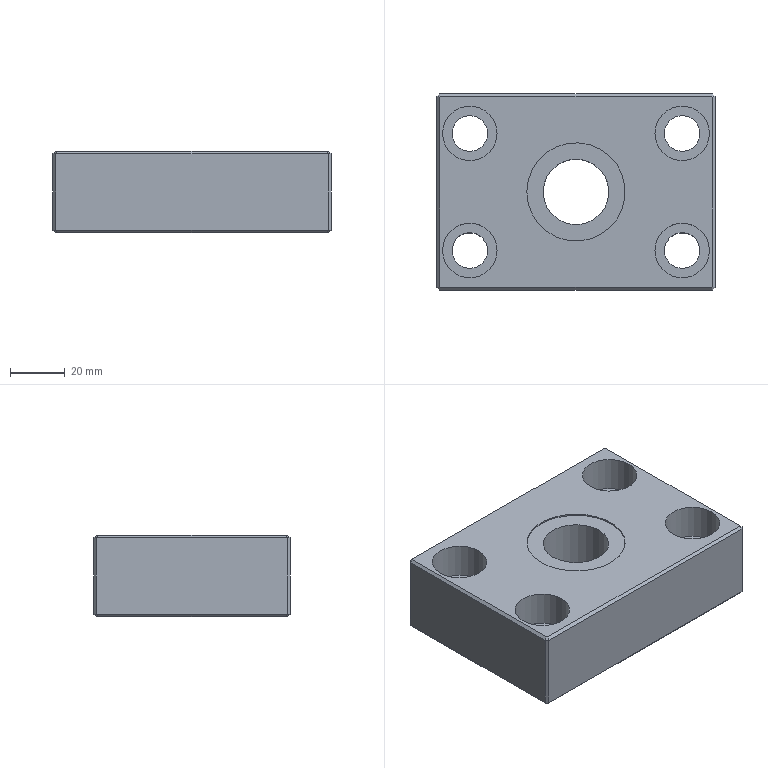Part | NX | 1 solid | 45 faces | box 102 x 72 x 30 mm | volume 178406 mm3 | plane 33 | cylinder 12 | commonest cylinder face diameters 13 x4 20 x4 24 x1 36 x1 54.5 x1 63.5 x1
STEP:
#1=CARTESIAN_POINT('',(31.75,0.,-27.25));
#2=VERTEX_POINT('',#1);
#3=CARTESIAN_POINT('',(0.,0.,-27.25));
#4=DIRECTION('',(0.,0.,-1.));
#5=DIRECTION('',(1.,0.,0.));
#6=AXIS2_PLACEMENT_3D('',#3,#4,#5);
#7=CIRCLE('',#6,31.75);
#8=EDGE_CURVE('',#2,#2,#7,.T.);
#9=ORIENTED_EDGE('',*,*,#8,.F.);
#10=EDGE_LOOP('',(#9));
#11=FACE_BOUND('',#10,.T.);
#12=CARTESIAN_POINT('',(-31.75,0.,-30.));
#13=VERTEX_POINT('',#12);
#14=CARTESIAN_POINT('',(0.,0.,-30.));
#15=DIRECTION('',(0.,0.,1.));
#16=DIRECTION('',(-1.,0.,0.));
#17=AXIS2_PLACEMENT_3D('',#14,#15,#16);
#18=CIRCLE('',#17,31.75);
#19=EDGE_CURVE('',#13,#13,#18,.T.);
#20=ORIENTED_EDGE('',*,*,#19,.F.);
#21=EDGE_LOOP('',(#20));
#22=FACE_BOUND('',#21,.T.);
#23=CARTESIAN_POINT('',(0.,0.,-27.25));
#24=DIRECTION('',(0.,0.,-1.));
#25=DIRECTION('',(-1.,0.,0.));
#26=AXIS2_PLACEMENT_3D('',#23,#24,#25);
#27=CYLINDRICAL_SURFACE('',#26,31.75);
#28=ADVANCED_FACE('',(#11,#22),#27,.F.);
#29=CARTESIAN_POINT('',(-27.25,0.,-27.25));
#30=VERTEX_POINT('',#29);
#31=CARTESIAN_POINT('',(0.,0.,-27.25));
#32=DIRECTION('',(0.,0.,-1.));
#33=DIRECTION('',(-1.,0.,0.));
#34=AXIS2_PLACEMENT_3D('',#31,#32,#33);
#35=CIRCLE('',#34,27.25);
#36=EDGE_CURVE('',#30,#30,#35,.T.);
#37=ORIENTED_EDGE('',*,*,#36,.T.);
#38=EDGE_LOOP('',(#37));
#39=FACE_BOUND('',#38,.T.);
#40=CARTESIAN_POINT('',(-27.25,0.,-30.));
#41=VERTEX_POINT('',#40);
#42=CARTESIAN_POINT('',(0.,0.,-30.));
#43=DIRECTION('',(0.,0.,1.));
#44=DIRECTION('',(-1.,0.,0.));
#45=AXIS2_PLACEMENT_3D('',#42,#43,#44);
#46=CIRCLE('',#45,27.25);
#47=EDGE_CURVE('',#41,#41,#46,.T.);
#48=ORIENTED_EDGE('',*,*,#47,.T.);
#49=EDGE_LOOP('',(#48));
#50=FACE_BOUND('',#49,.T.);
#51=CARTESIAN_POINT('',(0.,0.,-27.25));
#52=DIRECTION('',(0.,0.,-1.));
#53=DIRECTION('',(-1.,0.,0.));
#54=AXIS2_PLACEMENT_3D('',#51,#52,#53);
#55=CYLINDRICAL_SURFACE('',#54,27.25);
#56=ADVANCED_FACE('',(#39,#50),#55,.T.);
#57=ORIENTED_EDGE('',*,*,#8,.T.);
#58=EDGE_LOOP('',(#57));
#59=FACE_BOUND('',#58,.T.);
#60=ORIENTED_EDGE('',*,*,#36,.F.);
#61=EDGE_LOOP('',(#60));
#62=FACE_BOUND('',#61,.T.);
#63=CARTESIAN_POINT('',(0.,0.,-27.25));
#64=DIRECTION('',(0.,0.,-1.));
#65=DIRECTION('',(-1.,0.,0.));
#66=AXIS2_PLACEMENT_3D('',#63,#64,#65);
#67=PLANE('',#66);
#68=ADVANCED_FACE('',(#59,#62),#67,.T.);
#69=CARTESIAN_POINT('',(50.,-34.586,-30.));
#70=VERTEX_POINT('',#69);
#71=CARTESIAN_POINT('',(51.,-35.,-29.));
#72=VERTEX_POINT('',#71);
#73=CARTESIAN_POINT('',(44.324,-32.235,-35.676));
#74=DIRECTION('',(0.6786,-0.2811,0.6786));
#75=VECTOR('',#74,1000.);
#76=LINE('',#73,#75);
#77=EDGE_CURVE('',#70,#72,#76,.T.);
#78=ORIENTED_EDGE('',*,*,#77,.T.);
#79=CARTESIAN_POINT('',(50.,-36.,-29.));
#80=VERTEX_POINT('',#79);
#81=CARTESIAN_POINT('',(50.,-36.,-29.));
#82=DIRECTION('',(0.7071,0.7071,0.));
#83=VECTOR('',#82,1000.);
#84=LINE('',#81,#83);
#85=EDGE_CURVE('',#80,#72,#84,.T.);
#86=ORIENTED_EDGE('',*,*,#85,.F.);
#87=CARTESIAN_POINT('',(49.586,-35.,-30.));
#88=VERTEX_POINT('',#87);
#89=CARTESIAN_POINT('',(46.05,-26.463,-38.537));
#90=DIRECTION('',(-0.2811,0.6786,-0.6786));
#91=VECTOR('',#90,1000.);
#92=LINE('',#89,#91);
#93=EDGE_CURVE('',#80,#88,#92,.T.);
#94=ORIENTED_EDGE('',*,*,#93,.T.);
#95=CARTESIAN_POINT('',(42.293,-42.293,-30.));
#96=DIRECTION('',(-0.7071,-0.7071,0.));
#97=VECTOR('',#96,1000.);
#98=LINE('',#95,#97);
#99=EDGE_CURVE('',#70,#88,#98,.T.);
#100=ORIENTED_EDGE('',*,*,#99,.F.);
#101=EDGE_LOOP('',(#78,#86,#94,#100));
#102=FACE_BOUND('',#101,.T.);
#103=CARTESIAN_POINT('',(42.293,-42.293,-30.));
#104=DIRECTION('',(0.5,-0.5,-0.7071));
#105=DIRECTION('',(0.7071,0.7071,0.));
#106=AXIS2_PLACEMENT_3D('',#103,#104,#105);
#107=PLANE('',#106);
#108=ADVANCED_FACE('',(#102),#107,.T.);
#109=CARTESIAN_POINT('',(-50.,-36.,-29.));
#110=VERTEX_POINT('',#109);
#111=CARTESIAN_POINT('',(-49.586,-35.,-30.));
#112=VERTEX_POINT('',#111);
#113=CARTESIAN_POINT('',(-50.401,-36.967,-28.033));
#114=DIRECTION('',(0.2811,0.6786,-0.6786));
#115=VECTOR('',#114,1000.);
#116=LINE('',#113,#115);
#117=EDGE_CURVE('',#110,#112,#116,.T.);
#118=ORIENTED_EDGE('',*,*,#117,.T.);
#119=CARTESIAN_POINT('',(0.,-35.,-30.));
#120=DIRECTION('',(-1.,0.,0.));
#121=VECTOR('',#120,1000.);
#122=LINE('',#119,#121);
#123=EDGE_CURVE('',#88,#112,#122,.T.);
#124=ORIENTED_EDGE('',*,*,#123,.F.);
#125=ORIENTED_EDGE('',*,*,#93,.F.);
#126=CARTESIAN_POINT('',(0.,-36.,-29.));
#127=DIRECTION('',(1.,0.,0.));
#128=VECTOR('',#127,1000.);
#129=LINE('',#126,#128);
#130=EDGE_CURVE('',#110,#80,#129,.T.);
#131=ORIENTED_EDGE('',*,*,#130,.F.);
#132=EDGE_LOOP('',(#118,#124,#125,#131));
#133=FACE_BOUND('',#132,.T.);
#134=CARTESIAN_POINT('',(0.,-36.,-29.));
#135=DIRECTION('',(0.,0.7071,0.7071));
#136=DIRECTION('',(1.,0.,0.));
#137=AXIS2_PLACEMENT_3D('',#134,#135,#136);
#138=PLANE('',#137);
#139=ADVANCED_FACE('',(#133),#138,.F.);
#140=CARTESIAN_POINT('',(50.,34.586,-30.));
#141=VERTEX_POINT('',#140);
#142=CARTESIAN_POINT('',(51.,35.,-29.));
#143=VERTEX_POINT('',#142);
#144=CARTESIAN_POINT('',(44.324,32.235,-35.676));
#145=DIRECTION('',(0.6786,0.2811,0.6786));
#146=VECTOR('',#145,1000.);
#147=LINE('',#144,#146);
#148=EDGE_CURVE('',#141,#143,#147,.T.);
#149=ORIENTED_EDGE('',*,*,#148,.T.);
#150=CARTESIAN_POINT('',(51.,0.,-29.));
#151=DIRECTION('',(0.,1.,0.));
#152=VECTOR('',#151,1000.);
#153=LINE('',#150,#152);
#154=EDGE_CURVE('',#72,#143,#153,.T.);
#155=ORIENTED_EDGE('',*,*,#154,.F.);
#156=ORIENTED_EDGE('',*,*,#77,.F.);
#157=CARTESIAN_POINT('',(50.,0.,-30.));
#158=DIRECTION('',(0.,-1.,0.));
#159=VECTOR('',#158,1000.);
#160=LINE('',#157,#159);
#161=EDGE_CURVE('',#141,#70,#160,.T.);
#162=ORIENTED_EDGE('',*,*,#161,.F.);
#163=EDGE_LOOP('',(#149,#155,#156,#162));
#164=FACE_BOUND('',#163,.T.);
#165=CARTESIAN_POINT('',(51.,0.,-29.));
#166=DIRECTION('',(-0.7071,0.,0.7071));
#167=DIRECTION('',(0.,1.,0.));
#168=AXIS2_PLACEMENT_3D('',#165,#166,#167);
#169=PLANE('',#168);
#170=ADVANCED_FACE('',(#164),#169,.F.);
#171=CARTESIAN_POINT('',(-51.,-35.,-29.));
#172=VERTEX_POINT('',#171);
#173=CARTESIAN_POINT('',(-50.,-34.586,-30.));
#174=VERTEX_POINT('',#173);
#175=CARTESIAN_POINT('',(-44.324,-32.235,-35.676));
#176=DIRECTION('',(0.6786,0.2811,-0.6786));
#177=VECTOR('',#176,1000.);
#178=LINE('',#175,#177);
#179=EDGE_CURVE('',#172,#174,#178,.T.);
#180=ORIENTED_EDGE('',*,*,#179,.T.);
#181=CARTESIAN_POINT('',(-42.293,-42.293,-30.));
#182=DIRECTION('',(-0.7071,0.7071,0.));
#183=VECTOR('',#182,1000.);
#184=LINE('',#181,#183);
#185=EDGE_CURVE('',#112,#174,#184,.T.);
#186=ORIENTED_EDGE('',*,*,#185,.F.);
#187=ORIENTED_EDGE('',*,*,#117,.F.);
#188=CARTESIAN_POINT('',(-51.,-35.,-29.));
#189=DIRECTION('',(0.7071,-0.7071,0.));
#190=VECTOR('',#189,1000.);
#191=LINE('',#188,#190);
#192=EDGE_CURVE('',#172,#110,#191,.T.);
#193=ORIENTED_EDGE('',*,*,#192,.F.);
#194=EDGE_LOOP('',(#180,#186,#187,#193));
#195=FACE_BOUND('',#194,.T.);
#196=CARTESIAN_POINT('',(-42.293,-42.293,-30.));
#197=DIRECTION('',(-0.5,-0.5,-0.7071));
#198=DIRECTION('',(0.7071,-0.7071,0.));
#199=AXIS2_PLACEMENT_3D('',#196,#197,#198);
#200=PLANE('',#199);
#201=ADVANCED_FACE('',(#195),#200,.T.);
#202=CARTESIAN_POINT('',(49.586,35.,-30.));
#203=VERTEX_POINT('',#202);
#204=CARTESIAN_POINT('',(50.,36.,-29.));
#205=VERTEX_POINT('',#204);
#206=CARTESIAN_POINT('',(50.401,36.967,-28.033));
#207=DIRECTION('',(0.2811,0.6786,0.6786));
#208=VECTOR('',#207,1000.);
#209=LINE('',#206,#208);
#210=EDGE_CURVE('',#203,#205,#209,.T.);
#211=ORIENTED_EDGE('',*,*,#210,.T.);
#212=CARTESIAN_POINT('',(51.,35.,-29.));
#213=DIRECTION('',(-0.7071,0.7071,0.));
#214=VECTOR('',#213,1000.);
#215=LINE('',#212,#214);
#216=EDGE_CURVE('',#143,#205,#215,.T.);
#217=ORIENTED_EDGE('',*,*,#216,.F.);
#218=ORIENTED_EDGE('',*,*,#148,.F.);
#219=CARTESIAN_POINT('',(42.293,42.293,-30.));
#220=DIRECTION('',(0.7071,-0.7071,0.));
#221=VECTOR('',#220,1000.);
#222=LINE('',#219,#221);
#223=EDGE_CURVE('',#203,#141,#222,.T.);
#224=ORIENTED_EDGE('',*,*,#223,.F.);
#225=EDGE_LOOP('',(#211,#217,#218,#224));
#226=FACE_BOUND('',#225,.T.);
#227=CARTESIAN_POINT('',(42.293,42.293,-30.));
#228=DIRECTION('',(0.5,0.5,-0.7071));
#229=DIRECTION('',(-0.7071,0.7071,0.));
#230=AXIS2_PLACEMENT_3D('',#227,#228,#229);
#231=PLANE('',#230);
#232=ADVANCED_FACE('',(#226),#231,.T.);
#233=CARTESIAN_POINT('',(-51.,35.,-29.));
#234=VERTEX_POINT('',#233);
#235=CARTESIAN_POINT('',(-50.,34.586,-30.));
#236=VERTEX_POINT('',#235);
#237=CARTESIAN_POINT('',(-47.921,33.725,-32.079));
#238=DIRECTION('',(0.6786,-0.2811,-0.6786));
#239=VECTOR('',#238,1000.);
#240=LINE('',#237,#239);
#241=EDGE_CURVE('',#234,#236,#240,.T.);
#242=ORIENTED_EDGE('',*,*,#241,.T.);
#243=CARTESIAN_POINT('',(-50.,0.,-30.));
#244=DIRECTION('',(0.,1.,0.));
#245=VECTOR('',#244,1000.);
#246=LINE('',#243,#245);
#247=EDGE_CURVE('',#174,#236,#246,.T.);
#248=ORIENTED_EDGE('',*,*,#247,.F.);
#249=ORIENTED_EDGE('',*,*,#179,.F.);
#250=CARTESIAN_POINT('',(-51.,0.,-29.));
#251=DIRECTION('',(0.,-1.,0.));
#252=VECTOR('',#251,1000.);
#253=LINE('',#250,#252);
#254=EDGE_CURVE('',#234,#172,#253,.T.);
#255=ORIENTED_EDGE('',*,*,#254,.F.);
#256=EDGE_LOOP('',(#242,#248,#249,#255));
#257=FACE_BOUND('',#256,.T.);
#258=CARTESIAN_POINT('',(-51.,0.,-29.));
#259=DIRECTION('',(0.7071,0.,0.7071));
#260=DIRECTION('',(0.,-1.,0.));
#261=AXIS2_PLACEMENT_3D('',#258,#259,#260);
#262=PLANE('',#261);
#263=ADVANCED_FACE('',(#257),#262,.F.);
#264=CARTESIAN_POINT('',(-49.586,35.,-30.));
#265=VERTEX_POINT('',#264);
#266=CARTESIAN_POINT('',(-50.,36.,-29.));
#267=VERTEX_POINT('',#266);
#268=CARTESIAN_POINT('',(-46.05,26.463,-38.537));
#269=DIRECTION('',(-0.2811,0.6786,0.6786));
#270=VECTOR('',#269,1000.);
#271=LINE('',#268,#270);
#272=EDGE_CURVE('',#265,#267,#271,.T.);
#273=ORIENTED_EDGE('',*,*,#272,.T.);
#274=CARTESIAN_POINT('',(0.,36.,-29.));
#275=DIRECTION('',(-1.,0.,0.));
#276=VECTOR('',#275,1000.);
#277=LINE('',#274,#276);
#278=EDGE_CURVE('',#205,#267,#277,.T.);
#279=ORIENTED_EDGE('',*,*,#278,.F.);
#280=ORIENTED_EDGE('',*,*,#210,.F.);
#281=CARTESIAN_POINT('',(0.,35.,-30.));
#282=DIRECTION('',(1.,0.,0.));
#283=VECTOR('',#282,1000.);
#284=LINE('',#281,#283);
#285=EDGE_CURVE('',#265,#203,#284,.T.);
#286=ORIENTED_EDGE('',*,*,#285,.F.);
#287=EDGE_LOOP('',(#273,#279,#280,#286));
#288=FACE_BOUND('',#287,.T.);
#289=CARTESIAN_POINT('',(0.,36.,-29.));
#290=DIRECTION('',(0.,-0.7071,0.7071));
#291=DIRECTION('',(-1.,0.,0.));
#292=AXIS2_PLACEMENT_3D('',#289,#290,#291);
#293=PLANE('',#292);
#294=ADVANCED_FACE('',(#288),#293,.F.);
#295=ORIENTED_EDGE('',*,*,#241,.F.);
#296=CARTESIAN_POINT('',(-50.,36.,-29.));
#297=DIRECTION('',(-0.7071,-0.7071,0.));
#298=VECTOR('',#297,1000.);
#299=LINE('',#296,#298);
#300=EDGE_CURVE('',#267,#234,#299,.T.);
#301=ORIENTED_EDGE('',*,*,#300,.F.);
#302=ORIENTED_EDGE('',*,*,#272,.F.);
#303=CARTESIAN_POINT('',(-42.293,42.293,-30.));
#304=DIRECTION('',(0.7071,0.7071,0.));
#305=VECTOR('',#304,1000.);
#306=LINE('',#303,#305);
#307=EDGE_CURVE('',#236,#265,#306,.T.);
#308=ORIENTED_EDGE('',*,*,#307,.F.);
#309=EDGE_LOOP('',(#295,#301,#302,#308));
#310=FACE_BOUND('',#309,.T.);
#311=CARTESIAN_POINT('',(-42.293,42.293,-30.));
#312=DIRECTION('',(-0.5,0.5,-0.7071));
#313=DIRECTION('',(-0.7071,-0.7071,0.));
#314=AXIS2_PLACEMENT_3D('',#311,#312,#313);
#315=PLANE('',#314);
#316=ADVANCED_FACE('',(#310),#315,.T.);
#317=CARTESIAN_POINT('',(-49.586,35.,0.));
#318=VERTEX_POINT('',#317);
#319=CARTESIAN_POINT('',(-50.,36.,-1.));
#320=VERTEX_POINT('',#319);
#321=CARTESIAN_POINT('',(-46.05,26.463,8.537));
#322=DIRECTION('',(-0.2811,0.6786,-0.6786));
#323=VECTOR('',#322,1000.);
#324=LINE('',#321,#323);
#325=EDGE_CURVE('',#318,#320,#324,.T.);
#326=ORIENTED_EDGE('',*,*,#325,.T.);
#327=CARTESIAN_POINT('',(-51.,35.,-1.));
#328=VERTEX_POINT('',#327);
#329=CARTESIAN_POINT('',(-50.,36.,-1.));
#330=DIRECTION('',(0.7071,0.7071,0.));
#331=VECTOR('',#330,1000.);
#332=LINE('',#329,#331);
#333=EDGE_CURVE('',#328,#320,#332,.T.);
#334=ORIENTED_EDGE('',*,*,#333,.F.);
#335=CARTESIAN_POINT('',(-50.,34.586,0.));
#336=VERTEX_POINT('',#335);
#337=CARTESIAN_POINT('',(-44.324,32.235,5.676));
#338=DIRECTION('',(0.6786,-0.2811,0.6786));
#339=VECTOR('',#338,1000.);
#340=LINE('',#337,#339);
#341=EDGE_CURVE('',#328,#336,#340,.T.);
#342=ORIENTED_EDGE('',*,*,#341,.T.);
#343=CARTESIAN_POINT('',(-42.293,42.293,0.));
#344=DIRECTION('',(-0.7071,-0.7071,0.));
#345=VECTOR('',#344,1000.);
#346=LINE('',#343,#345);
#347=EDGE_CURVE('',#318,#336,#346,.T.);
#348=ORIENTED_EDGE('',*,*,#347,.F.);
#349=EDGE_LOOP('',(#326,#334,#342,#348));
#350=FACE_BOUND('',#349,.T.);
#351=CARTESIAN_POINT('',(-42.293,42.293,0.));
#352=DIRECTION('',(-0.5,0.5,0.7071));
#353=DIRECTION('',(0.7071,0.7071,0.));
#354=AXIS2_PLACEMENT_3D('',#351,#352,#353);
#355=PLANE('',#354);
#356=ADVANCED_FACE('',(#350),#355,.T.);
#357=CARTESIAN_POINT('',(-51.,-35.,-1.));
#358=VERTEX_POINT('',#357);
#359=CARTESIAN_POINT('',(-50.,-34.586,0.));
#360=VERTEX_POINT('',#359);
#361=CARTESIAN_POINT('',(-47.921,-33.725,2.079));
#362=DIRECTION('',(0.6786,0.2811,0.6786));
#363=VECTOR('',#362,1000.);
#364=LINE('',#361,#363);
#365=EDGE_CURVE('',#358,#360,#364,.T.);
#366=ORIENTED_EDGE('',*,*,#365,.T.);
#367=CARTESIAN_POINT('',(-50.,0.,0.));
#368=DIRECTION('',(0.,-1.,0.));
#369=VECTOR('',#368,1000.);
#370=LINE('',#367,#369);
#371=EDGE_CURVE('',#336,#360,#370,.T.);
#372=ORIENTED_EDGE('',*,*,#371,.F.);
#373=ORIENTED_EDGE('',*,*,#341,.F.);
#374=CARTESIAN_POINT('',(-51.,0.,-1.));
#375=DIRECTION('',(0.,1.,0.));
#376=VECTOR('',#375,1000.);
#377=LINE('',#374,#376);
#378=EDGE_CURVE('',#358,#328,#377,.T.);
#379=ORIENTED_EDGE('',*,*,#378,.F.);
#380=EDGE_LOOP('',(#366,#372,#373,#379));
#381=FACE_BOUND('',#380,.T.);
#382=CARTESIAN_POINT('',(-51.,0.,-1.));
#383=DIRECTION('',(0.7071,0.,-0.7071));
#384=DIRECTION('',(0.,1.,0.));
#385=AXIS2_PLACEMENT_3D('',#382,#383,#384);
#386=PLANE('',#385);
#387=ADVANCED_FACE('',(#381),#386,.F.);
#388=CARTESIAN_POINT('',(49.586,35.,0.));
#389=VERTEX_POINT('',#388);
#390=CARTESIAN_POINT('',(50.,36.,-1.));
#391=VERTEX_POINT('',#390);
#392=CARTESIAN_POINT('',(46.05,26.463,8.537));
#393=DIRECTION('',(0.2811,0.6786,-0.6786));
#394=VECTOR('',#393,1000.);
#395=LINE('',#392,#394);
#396=EDGE_CURVE('',#389,#391,#395,.T.);
#397=ORIENTED_EDGE('',*,*,#396,.T.);
#398=CARTESIAN_POINT('',(0.,36.,-1.));
#399=DIRECTION('',(1.,0.,0.));
#400=VECTOR('',#399,1000.);
#401=LINE('',#398,#400);
#402=EDGE_CURVE('',#320,#391,#401,.T.);
#403=ORIENTED_EDGE('',*,*,#402,.F.);
#404=ORIENTED_EDGE('',*,*,#325,.F.);
#405=CARTESIAN_POINT('',(0.,35.,0.));
#406=DIRECTION('',(-1.,0.,0.));
#407=VECTOR('',#406,1000.);
#408=LINE('',#405,#407);
#409=EDGE_CURVE('',#389,#318,#408,.T.);
#410=ORIENTED_EDGE('',*,*,#409,.F.);
#411=EDGE_LOOP('',(#397,#403,#404,#410));
#412=FACE_BOUND('',#411,.T.);
#413=CARTESIAN_POINT('',(0.,36.,-1.));
#414=DIRECTION('',(0.,-0.7071,-0.7071));
#415=DIRECTION('',(1.,0.,0.));
#416=AXIS2_PLACEMENT_3D('',#413,#414,#415);
#417=PLANE('',#416);
#418=ADVANCED_FACE('',(#412),#417,.F.);
#419=CARTESIAN_POINT('',(-50.,-36.,-1.));
#420=VERTEX_POINT('',#419);
#421=CARTESIAN_POINT('',(-49.586,-35.,0.));
#422=VERTEX_POINT('',#421);
#423=CARTESIAN_POINT('',(-46.05,-26.463,8.537));
#424=DIRECTION('',(0.2811,0.6786,0.6786));
#425=VECTOR('',#424,1000.);
#426=LINE('',#423,#425);
#427=EDGE_CURVE('',#420,#422,#426,.T.);
#428=ORIENTED_EDGE('',*,*,#427,.T.);
#429=CARTESIAN_POINT('',(-42.293,-42.293,0.));
#430=DIRECTION('',(0.7071,-0.7071,0.));
#431=VECTOR('',#430,1000.);
#432=LINE('',#429,#431);
#433=EDGE_CURVE('',#360,#422,#432,.T.);
#434=ORIENTED_EDGE('',*,*,#433,.F.);
#435=ORIENTED_EDGE('',*,*,#365,.F.);
#436=CARTESIAN_POINT('',(-51.,-35.,-1.));
#437=DIRECTION('',(-0.7071,0.7071,0.));
#438=VECTOR('',#437,1000.);
#439=LINE('',#436,#438);
#440=EDGE_CURVE('',#420,#358,#439,.T.);
#441=ORIENTED_EDGE('',*,*,#440,.F.);
#442=EDGE_LOOP('',(#428,#434,#435,#441));
#443=FACE_BOUND('',#442,.T.);
#444=CARTESIAN_POINT('',(-42.293,-42.293,0.));
#445=DIRECTION('',(-0.5,-0.5,0.7071));
#446=DIRECTION('',(-0.7071,0.7071,0.));
#447=AXIS2_PLACEMENT_3D('',#444,#445,#446);
#448=PLANE('',#447);
#449=ADVANCED_FACE('',(#443),#448,.T.);
#450=CARTESIAN_POINT('',(50.,34.586,0.));
#451=VERTEX_POINT('',#450);
#452=CARTESIAN_POINT('',(51.,35.,-1.));
#453=VERTEX_POINT('',#452);
#454=CARTESIAN_POINT('',(47.921,33.725,2.079));
#455=DIRECTION('',(0.6786,0.2811,-0.6786));
#456=VECTOR('',#455,1000.);
#457=LINE('',#454,#456);
#458=EDGE_CURVE('',#451,#453,#457,.T.);
#459=ORIENTED_EDGE('',*,*,#458,.T.);
#460=CARTESIAN_POINT('',(51.,35.,-1.));
#461=DIRECTION('',(0.7071,-0.7071,0.));
#462=VECTOR('',#461,1000.);
#463=LINE('',#460,#462);
#464=EDGE_CURVE('',#391,#453,#463,.T.);
#465=ORIENTED_EDGE('',*,*,#464,.F.);
#466=ORIENTED_EDGE('',*,*,#396,.F.);
#467=CARTESIAN_POINT('',(42.293,42.293,0.));
#468=DIRECTION('',(-0.7071,0.7071,0.));
#469=VECTOR('',#468,1000.);
#470=LINE('',#467,#469);
#471=EDGE_CURVE('',#451,#389,#470,.T.);
#472=ORIENTED_EDGE('',*,*,#471,.F.);
#473=EDGE_LOOP('',(#459,#465,#466,#472));
#474=FACE_BOUND('',#473,.T.);
#475=CARTESIAN_POINT('',(42.293,42.293,0.));
#476=DIRECTION('',(0.5,0.5,0.7071));
#477=DIRECTION('',(0.7071,-0.7071,0.));
#478=AXIS2_PLACEMENT_3D('',#475,#476,#477);
#479=PLANE('',#478);
#480=ADVANCED_FACE('',(#474),#479,.T.);
#481=CARTESIAN_POINT('',(50.,-36.,-1.));
#482=VERTEX_POINT('',#481);
#483=CARTESIAN_POINT('',(49.586,-35.,0.));
#484=VERTEX_POINT('',#483);
#485=CARTESIAN_POINT('',(50.401,-36.967,-1.967));
#486=DIRECTION('',(-0.2811,0.6786,0.6786));
#487=VECTOR('',#486,1000.);
#488=LINE('',#485,#487);
#489=EDGE_CURVE('',#482,#484,#488,.T.);
#490=ORIENTED_EDGE('',*,*,#489,.T.);
#491=CARTESIAN_POINT('',(0.,-35.,0.));
#492=DIRECTION('',(1.,0.,0.));
#493=VECTOR('',#492,1000.);
#494=LINE('',#491,#493);
#495=EDGE_CURVE('',#422,#484,#494,.T.);
#496=ORIENTED_EDGE('',*,*,#495,.F.);
#497=ORIENTED_EDGE('',*,*,#427,.F.);
#498=CARTESIAN_POINT('',(0.,-36.,-1.));
#499=DIRECTION('',(-1.,0.,0.));
#500=VECTOR('',#499,1000.);
#501=LINE('',#498,#500);
#502=EDGE_CURVE('',#482,#420,#501,.T.);
#503=ORIENTED_EDGE('',*,*,#502,.F.);
#504=EDGE_LOOP('',(#490,#496,#497,#503));
#505=FACE_BOUND('',#504,.T.);
#506=CARTESIAN_POINT('',(0.,-36.,-1.));
#507=DIRECTION('',(0.,0.7071,-0.7071));
#508=DIRECTION('',(-1.,0.,0.));
#509=AXIS2_PLACEMENT_3D('',#506,#507,#508);
#510=PLANE('',#509);
#511=ADVANCED_FACE('',(#505),#510,.F.);
#512=CARTESIAN_POINT('',(50.,-34.586,0.));
#513=VERTEX_POINT('',#512);
#514=CARTESIAN_POINT('',(51.,-35.,-1.));
#515=VERTEX_POINT('',#514);
#516=CARTESIAN_POINT('',(44.324,-32.235,5.676));
#517=DIRECTION('',(0.6786,-0.2811,-0.6786));
#518=VECTOR('',#517,1000.);
#519=LINE('',#516,#518);
#520=EDGE_CURVE('',#513,#515,#519,.T.);
#521=ORIENTED_EDGE('',*,*,#520,.T.);
#522=CARTESIAN_POINT('',(51.,0.,-1.));
#523=DIRECTION('',(0.,-1.,0.));
#524=VECTOR('',#523,1000.);
#525=LINE('',#522,#524);
#526=EDGE_CURVE('',#453,#515,#525,.T.);
#527=ORIENTED_EDGE('',*,*,#526,.F.);
#528=ORIENTED_EDGE('',*,*,#458,.F.);
#529=CARTESIAN_POINT('',(50.,0.,0.));
#530=DIRECTION('',(0.,1.,0.));
#531=VECTOR('',#530,1000.);
#532=LINE('',#529,#531);
#533=EDGE_CURVE('',#513,#451,#532,.T.);
#534=ORIENTED_EDGE('',*,*,#533,.F.);
#535=EDGE_LOOP('',(#521,#527,#528,#534));
#536=FACE_BOUND('',#535,.T.);
#537=CARTESIAN_POINT('',(51.,0.,-1.));
#538=DIRECTION('',(-0.7071,0.,-0.7071));
#539=DIRECTION('',(0.,-1.,0.));
#540=AXIS2_PLACEMENT_3D('',#537,#538,#539);
#541=PLANE('',#540);
#542=ADVANCED_FACE('',(#536),#541,.F.);
#543=ORIENTED_EDGE('',*,*,#489,.F.);
#544=CARTESIAN_POINT('',(50.,-36.,-1.));
#545=DIRECTION('',(-0.7071,-0.7071,0.));
#546=VECTOR('',#545,1000.);
#547=LINE('',#544,#546);
#548=EDGE_CURVE('',#515,#482,#547,.T.);
#549=ORIENTED_EDGE('',*,*,#548,.F.);
#550=ORIENTED_EDGE('',*,*,#520,.F.);
#551=CARTESIAN_POINT('',(42.293,-42.293,0.));
#552=DIRECTION('',(0.7071,0.7071,0.));
#553=VECTOR('',#552,1000.);
#554=LINE('',#551,#553);
#555=EDGE_CURVE('',#484,#513,#554,.T.);
#556=ORIENTED_EDGE('',*,*,#555,.F.);
#557=EDGE_LOOP('',(#543,#549,#550,#556));
#558=FACE_BOUND('',#557,.T.);
#559=CARTESIAN_POINT('',(42.293,-42.293,0.));
#560=DIRECTION('',(0.5,-0.5,0.7071));
#561=DIRECTION('',(-0.7071,-0.7071,0.));
#562=AXIS2_PLACEMENT_3D('',#559,#560,#561);
#563=PLANE('',#562);
#564=ADVANCED_FACE('',(#558),#563,.T.);
#565=CARTESIAN_POINT('',(50.,-36.,-30.));
#566=DIRECTION('',(0.,0.,1.));
#567=VECTOR('',#566,1000.);
#568=LINE('',#565,#567);
#569=EDGE_CURVE('',#80,#482,#568,.T.);
#570=ORIENTED_EDGE('',*,*,#569,.F.);
#571=ORIENTED_EDGE('',*,*,#85,.T.);
#572=CARTESIAN_POINT('',(51.,-35.,-30.));
#573=DIRECTION('',(0.,0.,-1.));
#574=VECTOR('',#573,1000.);
#575=LINE('',#572,#574);
#576=EDGE_CURVE('',#515,#72,#575,.T.);
#577=ORIENTED_EDGE('',*,*,#576,.F.);
#578=ORIENTED_EDGE('',*,*,#548,.T.);
#579=EDGE_LOOP('',(#570,#571,#577,#578));
#580=FACE_BOUND('',#579,.T.);
#581=CARTESIAN_POINT('',(50.,-36.,-30.));
#582=DIRECTION('',(-0.7071,0.7071,0.));
#583=DIRECTION('',(0.,0.,1.));
#584=AXIS2_PLACEMENT_3D('',#581,#582,#583);
#585=PLANE('',#584);
#586=ADVANCED_FACE('',(#580),#585,.F.);
#587=CARTESIAN_POINT('',(-51.,-35.,-30.));
#588=DIRECTION('',(0.,0.,1.));
#589=VECTOR('',#588,1000.);
#590=LINE('',#587,#589);
#591=EDGE_CURVE('',#172,#358,#590,.T.);
#592=ORIENTED_EDGE('',*,*,#591,.F.);
#593=ORIENTED_EDGE('',*,*,#192,.T.);
#594=CARTESIAN_POINT('',(-50.,-36.,-30.));
#595=DIRECTION('',(0.,0.,-1.));
#596=VECTOR('',#595,1000.);
#597=LINE('',#594,#596);
#598=EDGE_CURVE('',#420,#110,#597,.T.);
#599=ORIENTED_EDGE('',*,*,#598,.F.);
#600=ORIENTED_EDGE('',*,*,#440,.T.);
#601=EDGE_LOOP('',(#592,#593,#599,#600));
#602=FACE_BOUND('',#601,.T.);
#603=CARTESIAN_POINT('',(-51.,-35.,-30.));
#604=DIRECTION('',(0.7071,0.7071,0.));
#605=DIRECTION('',(0.,0.,1.));
#606=AXIS2_PLACEMENT_3D('',#603,#604,#605);
#607=PLANE('',#606);
#608=ADVANCED_FACE('',(#602),#607,.F.);
#609=CARTESIAN_POINT('',(51.,35.,-30.));
#610=DIRECTION('',(0.,0.,1.));
#611=VECTOR('',#610,1000.);
#612=LINE('',#609,#611);
#613=EDGE_CURVE('',#143,#453,#612,.T.);
#614=ORIENTED_EDGE('',*,*,#613,.F.);
#615=ORIENTED_EDGE('',*,*,#216,.T.);
#616=CARTESIAN_POINT('',(50.,36.,-30.));
#617=DIRECTION('',(0.,0.,-1.));
#618=VECTOR('',#617,1000.);
#619=LINE('',#616,#618);
#620=EDGE_CURVE('',#391,#205,#619,.T.);
#621=ORIENTED_EDGE('',*,*,#620,.F.);
#622=ORIENTED_EDGE('',*,*,#464,.T.);
#623=EDGE_LOOP('',(#614,#615,#621,#622));
#624=FACE_BOUND('',#623,.T.);
#625=CARTESIAN_POINT('',(51.,35.,-30.));
#626=DIRECTION('',(-0.7071,-0.7071,0.));
#627=DIRECTION('',(0.,0.,1.));
#628=AXIS2_PLACEMENT_3D('',#625,#626,#627);
#629=PLANE('',#628);
#630=ADVANCED_FACE('',(#624),#629,.F.);
#631=CARTESIAN_POINT('',(-50.,36.,-30.));
#632=DIRECTION('',(0.,0.,1.));
#633=VECTOR('',#632,1000.);
#634=LINE('',#631,#633);
#635=EDGE_CURVE('',#267,#320,#634,.T.);
#636=ORIENTED_EDGE('',*,*,#635,.F.);
#637=ORIENTED_EDGE('',*,*,#300,.T.);
#638=CARTESIAN_POINT('',(-51.,35.,-30.));
#639=DIRECTION('',(0.,0.,-1.));
#640=VECTOR('',#639,1000.);
#641=LINE('',#638,#640);
#642=EDGE_CURVE('',#328,#234,#641,.T.);
#643=ORIENTED_EDGE('',*,*,#642,.F.);
#644=ORIENTED_EDGE('',*,*,#333,.T.);
#645=EDGE_LOOP('',(#636,#637,#643,#644));
#646=FACE_BOUND('',#645,.T.);
#647=CARTESIAN_POINT('',(-50.,36.,-30.));
#648=DIRECTION('',(0.7071,-0.7071,0.));
#649=DIRECTION('',(0.,0.,1.));
#650=AXIS2_PLACEMENT_3D('',#647,#648,#649);
#651=PLANE('',#650);
#652=ADVANCED_FACE('',(#646),#651,.F.);
#653=CARTESIAN_POINT('',(-18.,0.,0.));
#654=VERTEX_POINT('',#653);
#655=CARTESIAN_POINT('',(0.,0.,0.));
#656=DIRECTION('',(0.,0.,-1.));
#657=DIRECTION('',(-1.,0.,0.));
#658=AXIS2_PLACEMENT_3D('',#655,#656,#657);
#659=CIRCLE('',#658,18.);
#660=EDGE_CURVE('',#654,#654,#659,.T.);
#661=ORIENTED_EDGE('',*,*,#660,.F.);
#662=EDGE_LOOP('',(#661));
#663=FACE_BOUND('',#662,.T.);
#664=CARTESIAN_POINT('',(-18.,0.,-0.5));
#665=VERTEX_POINT('',#664);
#666=CARTESIAN_POINT('',(0.,0.,-0.5));
#667=DIRECTION('',(0.,0.,1.));
#668=DIRECTION('',(-1.,0.,0.));
#669=AXIS2_PLACEMENT_3D('',#666,#667,#668);
#670=CIRCLE('',#669,18.);
#671=EDGE_CURVE('',#665,#665,#670,.T.);
#672=ORIENTED_EDGE('',*,*,#671,.F.);
#673=EDGE_LOOP('',(#672));
#674=FACE_BOUND('',#673,.T.);
#675=CARTESIAN_POINT('',(0.,0.,0.));
#676=DIRECTION('',(0.,0.,-1.));
#677=DIRECTION('',(-1.,0.,0.));
#678=AXIS2_PLACEMENT_3D('',#675,#676,#677);
#679=CYLINDRICAL_SURFACE('',#678,18.);
#680=ADVANCED_FACE('',(#663,#674),#679,.F.);
#681=ORIENTED_EDGE('',*,*,#671,.T.);
#682=EDGE_LOOP('',(#681));
#683=FACE_BOUND('',#682,.T.);
#684=CARTESIAN_POINT('',(-12.,0.,-0.5));
#685=VERTEX_POINT('',#684);
#686=CARTESIAN_POINT('',(0.,0.,-0.5));
#687=DIRECTION('',(0.,0.,1.));
#688=DIRECTION('',(-1.,0.,0.));
#689=AXIS2_PLACEMENT_3D('',#686,#687,#688);
#690=CIRCLE('',#689,12.);
#691=EDGE_CURVE('',#685,#685,#690,.T.);
#692=ORIENTED_EDGE('',*,*,#691,.F.);
#693=EDGE_LOOP('',(#692));
#694=FACE_BOUND('',#693,.T.);
#695=CARTESIAN_POINT('',(0.,0.,-0.5));
#696=DIRECTION('',(0.,0.,-1.));
#697=DIRECTION('',(-1.,0.,0.));
#698=AXIS2_PLACEMENT_3D('',#695,#696,#697);
#699=PLANE('',#698);
#700=ADVANCED_FACE('',(#683,#694),#699,.F.);
#701=ORIENTED_EDGE('',*,*,#691,.T.);
#702=EDGE_LOOP('',(#701));
#703=FACE_BOUND('',#702,.T.);
#704=CARTESIAN_POINT('',(-12.,0.,-30.));
#705=VERTEX_POINT('',#704);
#706=CARTESIAN_POINT('',(0.,0.,-30.));
#707=DIRECTION('',(0.,0.,-1.));
#708=DIRECTION('',(-1.,0.,0.));
#709=AXIS2_PLACEMENT_3D('',#706,#707,#708);
#710=CIRCLE('',#709,12.);
#711=EDGE_CURVE('',#705,#705,#710,.T.);
#712=ORIENTED_EDGE('',*,*,#711,.T.);
#713=EDGE_LOOP('',(#712));
#714=FACE_BOUND('',#713,.T.);
#715=CARTESIAN_POINT('',(0.,0.,-50.));
#716=DIRECTION('',(0.,0.,-1.));
#717=DIRECTION('',(-1.,0.,0.));
#718=AXIS2_PLACEMENT_3D('',#715,#716,#717);
#719=CYLINDRICAL_SURFACE('',#718,12.);
#720=ADVANCED_FACE('',(#703,#714),#719,.F.);
#721=CARTESIAN_POINT('',(-48.9,21.45,0.));
#722=VERTEX_POINT('',#721);
#723=CARTESIAN_POINT('',(-38.9,21.45,0.));
#724=DIRECTION('',(0.,0.,-1.));
#725=DIRECTION('',(-1.,0.,0.));
#726=AXIS2_PLACEMENT_3D('',#723,#724,#725);
#727=CIRCLE('',#726,10.);
#728=EDGE_CURVE('',#722,#722,#727,.T.);
#729=ORIENTED_EDGE('',*,*,#728,.F.);
#730=EDGE_LOOP('',(#729));
#731=FACE_BOUND('',#730,.T.);
#732=CARTESIAN_POINT('',(-48.9,21.45,-13.));
#733=VERTEX_POINT('',#732);
#734=CARTESIAN_POINT('',(-38.9,21.45,-13.));
#735=DIRECTION('',(0.,0.,1.));
#736=DIRECTION('',(-1.,0.,0.));
#737=AXIS2_PLACEMENT_3D('',#734,#735,#736);
#738=CIRCLE('',#737,10.);
#739=EDGE_CURVE('',#733,#733,#738,.T.);
#740=ORIENTED_EDGE('',*,*,#739,.F.);
#741=EDGE_LOOP('',(#740));
#742=FACE_BOUND('',#741,.T.);
#743=CARTESIAN_POINT('',(-38.9,21.45,0.));
#744=DIRECTION('',(0.,0.,-1.));
#745=DIRECTION('',(-1.,0.,0.));
#746=AXIS2_PLACEMENT_3D('',#743,#744,#745);
#747=CYLINDRICAL_SURFACE('',#746,10.);
#748=ADVANCED_FACE('',(#731,#742),#747,.F.);
#749=ORIENTED_EDGE('',*,*,#739,.T.);
#750=EDGE_LOOP('',(#749));
#751=FACE_BOUND('',#750,.T.);
#752=CARTESIAN_POINT('',(-45.4,21.45,-13.));
#753=VERTEX_POINT('',#752);
#754=CARTESIAN_POINT('',(-38.9,21.45,-13.));
#755=DIRECTION('',(0.,0.,1.));
#756=DIRECTION('',(-1.,0.,0.));
#757=AXIS2_PLACEMENT_3D('',#754,#755,#756);
#758=CIRCLE('',#757,6.5);
#759=EDGE_CURVE('',#753,#753,#758,.T.);
#760=ORIENTED_EDGE('',*,*,#759,.F.);
#761=EDGE_LOOP('',(#760));
#762=FACE_BOUND('',#761,.T.);
#763=CARTESIAN_POINT('',(-38.9,21.45,-13.));
#764=DIRECTION('',(0.,0.,-1.));
#765=DIRECTION('',(-1.,0.,0.));
#766=AXIS2_PLACEMENT_3D('',#763,#764,#765);
#767=PLANE('',#766);
#768=ADVANCED_FACE('',(#751,#762),#767,.F.);
#769=ORIENTED_EDGE('',*,*,#759,.T.);
#770=EDGE_LOOP('',(#769));
#771=FACE_BOUND('',#770,.T.);
#772=CARTESIAN_POINT('',(-45.4,21.45,-30.));
#773=VERTEX_POINT('',#772);
#774=CARTESIAN_POINT('',(-38.9,21.45,-30.));
#775=DIRECTION('',(0.,0.,-1.));
#776=DIRECTION('',(-1.,0.,0.));
#777=AXIS2_PLACEMENT_3D('',#774,#775,#776);
#778=CIRCLE('',#777,6.5);
#779=EDGE_CURVE('',#773,#773,#778,.T.);
#780=ORIENTED_EDGE('',*,*,#779,.T.);
#781=EDGE_LOOP('',(#780));
#782=FACE_BOUND('',#781,.T.);
#783=CARTESIAN_POINT('',(-38.9,21.45,-50.));
#784=DIRECTION('',(0.,0.,-1.));
#785=DIRECTION('',(-1.,0.,0.));
#786=AXIS2_PLACEMENT_3D('',#783,#784,#785);
#787=CYLINDRICAL_SURFACE('',#786,6.5);
#788=ADVANCED_FACE('',(#771,#782),#787,.F.);
#789=ORIENTED_EDGE('',*,*,#576,.T.);
#790=ORIENTED_EDGE('',*,*,#154,.T.);
#791=ORIENTED_EDGE('',*,*,#613,.T.);
#792=ORIENTED_EDGE('',*,*,#526,.T.);
#793=EDGE_LOOP('',(#789,#790,#791,#792));
#794=FACE_BOUND('',#793,.T.);
#795=CARTESIAN_POINT('',(51.,0.,-30.));
#796=DIRECTION('',(1.,0.,0.));
#797=DIRECTION('',(0.,0.,-1.));
#798=AXIS2_PLACEMENT_3D('',#795,#796,#797);
#799=PLANE('',#798);
#800=ADVANCED_FACE('',(#794),#799,.T.);
#801=ORIENTED_EDGE('',*,*,#779,.F.);
#802=EDGE_LOOP('',(#801));
#803=FACE_BOUND('',#802,.T.);
#804=CARTESIAN_POINT('',(-45.4,-21.45,-30.));
#805=VERTEX_POINT('',#804);
#806=CARTESIAN_POINT('',(-38.9,-21.45,-30.));
#807=DIRECTION('',(0.,0.,-1.));
#808=DIRECTION('',(-1.,0.,0.));
#809=AXIS2_PLACEMENT_3D('',#806,#807,#808);
#810=CIRCLE('',#809,6.5);
#811=EDGE_CURVE('',#805,#805,#810,.T.);
#812=ORIENTED_EDGE('',*,*,#811,.F.);
#813=EDGE_LOOP('',(#812));
#814=FACE_BOUND('',#813,.T.);
#815=CARTESIAN_POINT('',(32.4,-21.45,-30.));
#816=VERTEX_POINT('',#815);
#817=CARTESIAN_POINT('',(38.9,-21.45,-30.));
#818=DIRECTION('',(0.,0.,-1.));
#819=DIRECTION('',(-1.,0.,0.));
#820=AXIS2_PLACEMENT_3D('',#817,#818,#819);
#821=CIRCLE('',#820,6.5);
#822=EDGE_CURVE('',#816,#816,#821,.T.);
#823=ORIENTED_EDGE('',*,*,#822,.F.);
#824=EDGE_LOOP('',(#823));
#825=FACE_BOUND('',#824,.T.);
#826=CARTESIAN_POINT('',(32.4,21.45,-30.));
#827=VERTEX_POINT('',#826);
#828=CARTESIAN_POINT('',(38.9,21.45,-30.));
#829=DIRECTION('',(0.,0.,-1.));
#830=DIRECTION('',(-1.,0.,0.));
#831=AXIS2_PLACEMENT_3D('',#828,#829,#830);
#832=CIRCLE('',#831,6.5);
#833=EDGE_CURVE('',#827,#827,#832,.T.);
#834=ORIENTED_EDGE('',*,*,#833,.F.);
#835=EDGE_LOOP('',(#834));
#836=FACE_BOUND('',#835,.T.);
#837=ORIENTED_EDGE('',*,*,#161,.T.);
#838=ORIENTED_EDGE('',*,*,#99,.T.);
#839=ORIENTED_EDGE('',*,*,#123,.T.);
#840=ORIENTED_EDGE('',*,*,#185,.T.);
#841=ORIENTED_EDGE('',*,*,#247,.T.);
#842=ORIENTED_EDGE('',*,*,#307,.T.);
#843=ORIENTED_EDGE('',*,*,#285,.T.);
#844=ORIENTED_EDGE('',*,*,#223,.T.);
#845=EDGE_LOOP('',(#837,#838,#839,#840,#841,#842,#843,#844));
#846=FACE_BOUND('',#845,.T.);
#847=ORIENTED_EDGE('',*,*,#19,.T.);
#848=EDGE_LOOP('',(#847));
#849=FACE_BOUND('',#848,.T.);
#850=CARTESIAN_POINT('',(0.,0.,-30.));
#851=DIRECTION('',(0.,0.,-1.));
#852=DIRECTION('',(-1.,0.,0.));
#853=AXIS2_PLACEMENT_3D('',#850,#851,#852);
#854=PLANE('',#853);
#855=ADVANCED_FACE('',(#803,#814,#825,#836,#846,#849),#854,.T.);
#856=ORIENTED_EDGE('',*,*,#620,.T.);
#857=ORIENTED_EDGE('',*,*,#278,.T.);
#858=ORIENTED_EDGE('',*,*,#635,.T.);
#859=ORIENTED_EDGE('',*,*,#402,.T.);
#860=EDGE_LOOP('',(#856,#857,#858,#859));
#861=FACE_BOUND('',#860,.T.);
#862=CARTESIAN_POINT('',(0.,36.,-30.));
#863=DIRECTION('',(0.,1.,0.));
#864=DIRECTION('',(0.,0.,1.));
#865=AXIS2_PLACEMENT_3D('',#862,#863,#864);
#866=PLANE('',#865);
#867=ADVANCED_FACE('',(#861),#866,.T.);
#868=ORIENTED_EDGE('',*,*,#642,.T.);
#869=ORIENTED_EDGE('',*,*,#254,.T.);
#870=ORIENTED_EDGE('',*,*,#591,.T.);
#871=ORIENTED_EDGE('',*,*,#378,.T.);
#872=EDGE_LOOP('',(#868,#869,#870,#871));
#873=FACE_BOUND('',#872,.T.);
#874=CARTESIAN_POINT('',(-51.,0.,-30.));
#875=DIRECTION('',(-1.,0.,0.));
#876=DIRECTION('',(0.,0.,1.));
#877=AXIS2_PLACEMENT_3D('',#874,#875,#876);
#878=PLANE('',#877);
#879=ADVANCED_FACE('',(#873),#878,.T.);
#880=ORIENTED_EDGE('',*,*,#598,.T.);
#881=ORIENTED_EDGE('',*,*,#130,.T.);
#882=ORIENTED_EDGE('',*,*,#569,.T.);
#883=ORIENTED_EDGE('',*,*,#502,.T.);
#884=EDGE_LOOP('',(#880,#881,#882,#883));
#885=FACE_BOUND('',#884,.T.);
#886=CARTESIAN_POINT('',(0.,-36.,-30.));
#887=DIRECTION('',(0.,-1.,0.));
#888=DIRECTION('',(0.,0.,-1.));
#889=AXIS2_PLACEMENT_3D('',#886,#887,#888);
#890=PLANE('',#889);
#891=ADVANCED_FACE('',(#885),#890,.T.);
#892=ORIENTED_EDGE('',*,*,#728,.T.);
#893=EDGE_LOOP('',(#892));
#894=FACE_BOUND('',#893,.T.);
#895=CARTESIAN_POINT('',(-48.9,-21.45,0.));
#896=VERTEX_POINT('',#895);
#897=CARTESIAN_POINT('',(-38.9,-21.45,0.));
#898=DIRECTION('',(0.,0.,-1.));
#899=DIRECTION('',(-1.,0.,0.));
#900=AXIS2_PLACEMENT_3D('',#897,#898,#899);
#901=CIRCLE('',#900,10.);
#902=EDGE_CURVE('',#896,#896,#901,.T.);
#903=ORIENTED_EDGE('',*,*,#902,.T.);
#904=EDGE_LOOP('',(#903));
#905=FACE_BOUND('',#904,.T.);
#906=CARTESIAN_POINT('',(28.9,-21.45,0.));
#907=VERTEX_POINT('',#906);
#908=CARTESIAN_POINT('',(38.9,-21.45,0.));
#909=DIRECTION('',(0.,0.,-1.));
#910=DIRECTION('',(-1.,0.,0.));
#911=AXIS2_PLACEMENT_3D('',#908,#909,#910);
#912=CIRCLE('',#911,10.);
#913=EDGE_CURVE('',#907,#907,#912,.T.);
#914=ORIENTED_EDGE('',*,*,#913,.T.);
#915=EDGE_LOOP('',(#914));
#916=FACE_BOUND('',#915,.T.);
#917=CARTESIAN_POINT('',(28.9,21.45,0.));
#918=VERTEX_POINT('',#917);
#919=CARTESIAN_POINT('',(38.9,21.45,0.));
#920=DIRECTION('',(0.,0.,-1.));
#921=DIRECTION('',(-1.,0.,0.));
#922=AXIS2_PLACEMENT_3D('',#919,#920,#921);
#923=CIRCLE('',#922,10.);
#924=EDGE_CURVE('',#918,#918,#923,.T.);
#925=ORIENTED_EDGE('',*,*,#924,.T.);
#926=EDGE_LOOP('',(#925));
#927=FACE_BOUND('',#926,.T.);
#928=ORIENTED_EDGE('',*,*,#660,.T.);
#929=EDGE_LOOP('',(#928));
#930=FACE_BOUND('',#929,.T.);
#931=ORIENTED_EDGE('',*,*,#409,.T.);
#932=ORIENTED_EDGE('',*,*,#347,.T.);
#933=ORIENTED_EDGE('',*,*,#371,.T.);
#934=ORIENTED_EDGE('',*,*,#433,.T.);
#935=ORIENTED_EDGE('',*,*,#495,.T.);
#936=ORIENTED_EDGE('',*,*,#555,.T.);
#937=ORIENTED_EDGE('',*,*,#533,.T.);
#938=ORIENTED_EDGE('',*,*,#471,.T.);
#939=EDGE_LOOP('',(#931,#932,#933,#934,#935,#936,#937,#938));
#940=FACE_BOUND('',#939,.T.);
#941=CARTESIAN_POINT('',(0.,0.,0.));
#942=DIRECTION('',(0.,0.,1.));
#943=DIRECTION('',(1.,0.,0.));
#944=AXIS2_PLACEMENT_3D('',#941,#942,#943);
#945=PLANE('',#944);
#946=ADVANCED_FACE('',(#894,#905,#916,#927,#930,#940),#945,.T.);
#947=ORIENTED_EDGE('',*,*,#902,.F.);
#948=EDGE_LOOP('',(#947));
#949=FACE_BOUND('',#948,.T.);
#950=CARTESIAN_POINT('',(-48.9,-21.45,-13.));
#951=VERTEX_POINT('',#950);
#952=CARTESIAN_POINT('',(-38.9,-21.45,-13.));
#953=DIRECTION('',(0.,0.,1.));
#954=DIRECTION('',(-1.,0.,0.));
#955=AXIS2_PLACEMENT_3D('',#952,#953,#954);
#956=CIRCLE('',#955,10.);
#957=EDGE_CURVE('',#951,#951,#956,.T.);
#958=ORIENTED_EDGE('',*,*,#957,.F.);
#959=EDGE_LOOP('',(#958));
#960=FACE_BOUND('',#959,.T.);
#961=CARTESIAN_POINT('',(-38.9,-21.45,0.));
#962=DIRECTION('',(0.,0.,-1.));
#963=DIRECTION('',(-1.,0.,0.));
#964=AXIS2_PLACEMENT_3D('',#961,#962,#963);
#965=CYLINDRICAL_SURFACE('',#964,10.);
#966=ADVANCED_FACE('',(#949,#960),#965,.F.);
#967=CARTESIAN_POINT('',(-45.4,-21.45,-13.));
#968=VERTEX_POINT('',#967);
#969=CARTESIAN_POINT('',(-38.9,-21.45,-13.));
#970=DIRECTION('',(0.,0.,1.));
#971=DIRECTION('',(-1.,0.,0.));
#972=AXIS2_PLACEMENT_3D('',#969,#970,#971);
#973=CIRCLE('',#972,6.5);
#974=EDGE_CURVE('',#968,#968,#973,.T.);
#975=ORIENTED_EDGE('',*,*,#974,.T.);
#976=EDGE_LOOP('',(#975));
#977=FACE_BOUND('',#976,.T.);
#978=ORIENTED_EDGE('',*,*,#811,.T.);
#979=EDGE_LOOP('',(#978));
#980=FACE_BOUND('',#979,.T.);
#981=CARTESIAN_POINT('',(-38.9,-21.45,-50.));
#982=DIRECTION('',(0.,0.,-1.));
#983=DIRECTION('',(-1.,0.,0.));
#984=AXIS2_PLACEMENT_3D('',#981,#982,#983);
#985=CYLINDRICAL_SURFACE('',#984,6.5);
#986=ADVANCED_FACE('',(#977,#980),#985,.F.);
#987=ORIENTED_EDGE('',*,*,#957,.T.);
#988=EDGE_LOOP('',(#987));
#989=FACE_BOUND('',#988,.T.);
#990=ORIENTED_EDGE('',*,*,#974,.F.);
#991=EDGE_LOOP('',(#990));
#992=FACE_BOUND('',#991,.T.);
#993=CARTESIAN_POINT('',(-38.9,-21.45,-13.));
#994=DIRECTION('',(0.,0.,-1.));
#995=DIRECTION('',(-1.,0.,0.));
#996=AXIS2_PLACEMENT_3D('',#993,#994,#995);
#997=PLANE('',#996);
#998=ADVANCED_FACE('',(#989,#992),#997,.F.);
#999=ORIENTED_EDGE('',*,*,#924,.F.);
#1000=EDGE_LOOP('',(#999));
#1001=FACE_BOUND('',#1000,.T.);
#1002=CARTESIAN_POINT('',(28.9,21.45,-13.));
#1003=VERTEX_POINT('',#1002);
#1004=CARTESIAN_POINT('',(38.9,21.45,-13.));
#1005=DIRECTION('',(0.,0.,1.));
#1006=DIRECTION('',(-1.,0.,0.));
#1007=AXIS2_PLACEMENT_3D('',#1004,#1005,#1006);
#1008=CIRCLE('',#1007,10.);
#1009=EDGE_CURVE('',#1003,#1003,#1008,.T.);
#1010=ORIENTED_EDGE('',*,*,#1009,.F.);
#1011=EDGE_LOOP('',(#1010));
#1012=FACE_BOUND('',#1011,.T.);
#1013=CARTESIAN_POINT('',(38.9,21.45,0.));
#1014=DIRECTION('',(0.,0.,-1.));
#1015=DIRECTION('',(-1.,0.,0.));
#1016=AXIS2_PLACEMENT_3D('',#1013,#1014,#1015);
#1017=CYLINDRICAL_SURFACE('',#1016,10.);
#1018=ADVANCED_FACE('',(#1001,#1012),#1017,.F.);
#1019=CARTESIAN_POINT('',(32.4,21.45,-13.));
#1020=VERTEX_POINT('',#1019);
#1021=CARTESIAN_POINT('',(38.9,21.45,-13.));
#1022=DIRECTION('',(0.,0.,1.));
#1023=DIRECTION('',(-1.,0.,0.));
#1024=AXIS2_PLACEMENT_3D('',#1021,#1022,#1023);
#1025=CIRCLE('',#1024,6.5);
#1026=EDGE_CURVE('',#1020,#1020,#1025,.T.);
#1027=ORIENTED_EDGE('',*,*,#1026,.T.);
#1028=EDGE_LOOP('',(#1027));
#1029=FACE_BOUND('',#1028,.T.);
#1030=ORIENTED_EDGE('',*,*,#833,.T.);
#1031=EDGE_LOOP('',(#1030));
#1032=FACE_BOUND('',#1031,.T.);
#1033=CARTESIAN_POINT('',(38.9,21.45,-50.));
#1034=DIRECTION('',(0.,0.,-1.));
#1035=DIRECTION('',(-1.,0.,0.));
#1036=AXIS2_PLACEMENT_3D('',#1033,#1034,#1035);
#1037=CYLINDRICAL_SURFACE('',#1036,6.5);
#1038=ADVANCED_FACE('',(#1029,#1032),#1037,.F.);
#1039=CARTESIAN_POINT('',(32.4,-21.45,-13.));
#1040=VERTEX_POINT('',#1039);
#1041=CARTESIAN_POINT('',(38.9,-21.45,-13.));
#1042=DIRECTION('',(0.,0.,1.));
#1043=DIRECTION('',(-1.,0.,0.));
#1044=AXIS2_PLACEMENT_3D('',#1041,#1042,#1043);
#1045=CIRCLE('',#1044,6.5);
#1046=EDGE_CURVE('',#1040,#1040,#1045,.T.);
#1047=ORIENTED_EDGE('',*,*,#1046,.T.);
#1048=EDGE_LOOP('',(#1047));
#1049=FACE_BOUND('',#1048,.T.);
#1050=ORIENTED_EDGE('',*,*,#822,.T.);
#1051=EDGE_LOOP('',(#1050));
#1052=FACE_BOUND('',#1051,.T.);
#1053=CARTESIAN_POINT('',(38.9,-21.45,-50.));
#1054=DIRECTION('',(0.,0.,-1.));
#1055=DIRECTION('',(-1.,0.,0.));
#1056=AXIS2_PLACEMENT_3D('',#1053,#1054,#1055);
#1057=CYLINDRICAL_SURFACE('',#1056,6.5);
#1058=ADVANCED_FACE('',(#1049,#1052),#1057,.F.);
#1059=ORIENTED_EDGE('',*,*,#1009,.T.);
#1060=EDGE_LOOP('',(#1059));
#1061=FACE_BOUND('',#1060,.T.);
#1062=ORIENTED_EDGE('',*,*,#1026,.F.);
#1063=EDGE_LOOP('',(#1062));
#1064=FACE_BOUND('',#1063,.T.);
#1065=CARTESIAN_POINT('',(38.9,21.45,-13.));
#1066=DIRECTION('',(0.,0.,-1.));
#1067=DIRECTION('',(-1.,0.,0.));
#1068=AXIS2_PLACEMENT_3D('',#1065,#1066,#1067);
#1069=PLANE('',#1068);
#1070=ADVANCED_FACE('',(#1061,#1064),#1069,.F.);
#1071=ORIENTED_EDGE('',*,*,#913,.F.);
#1072=EDGE_LOOP('',(#1071));
#1073=FACE_BOUND('',#1072,.T.);
#1074=CARTESIAN_POINT('',(28.9,-21.45,-13.));
#1075=VERTEX_POINT('',#1074);
#1076=CARTESIAN_POINT('',(38.9,-21.45,-13.));
#1077=DIRECTION('',(0.,0.,1.));
#1078=DIRECTION('',(-1.,0.,0.));
#1079=AXIS2_PLACEMENT_3D('',#1076,#1077,#1078);
#1080=CIRCLE('',#1079,10.);
#1081=EDGE_CURVE('',#1075,#1075,#1080,.T.);
#1082=ORIENTED_EDGE('',*,*,#1081,.F.);
#1083=EDGE_LOOP('',(#1082));
#1084=FACE_BOUND('',#1083,.T.);
#1085=CARTESIAN_POINT('',(38.9,-21.45,0.));
#1086=DIRECTION('',(0.,0.,-1.));
#1087=DIRECTION('',(-1.,0.,0.));
#1088=AXIS2_PLACEMENT_3D('',#1085,#1086,#1087);
#1089=CYLINDRICAL_SURFACE('',#1088,10.);
#1090=ADVANCED_FACE('',(#1073,#1084),#1089,.F.);
#1091=ORIENTED_EDGE('',*,*,#1081,.T.);
#1092=EDGE_LOOP('',(#1091));
#1093=FACE_BOUND('',#1092,.T.);
#1094=ORIENTED_EDGE('',*,*,#1046,.F.);
#1095=EDGE_LOOP('',(#1094));
#1096=FACE_BOUND('',#1095,.T.);
#1097=CARTESIAN_POINT('',(38.9,-21.45,-13.));
#1098=DIRECTION('',(0.,0.,-1.));
#1099=DIRECTION('',(-1.,0.,0.));
#1100=AXIS2_PLACEMENT_3D('',#1097,#1098,#1099);
#1101=PLANE('',#1100);
#1102=ADVANCED_FACE('',(#1093,#1096),#1101,.F.);
#1103=ORIENTED_EDGE('',*,*,#47,.F.);
#1104=EDGE_LOOP('',(#1103));
#1105=FACE_BOUND('',#1104,.T.);
#1106=ORIENTED_EDGE('',*,*,#711,.F.);
#1107=EDGE_LOOP('',(#1106));
#1108=FACE_BOUND('',#1107,.T.);
#1109=CARTESIAN_POINT('',(0.,0.,-30.));
#1110=DIRECTION('',(0.,0.,-1.));
#1111=DIRECTION('',(-1.,0.,0.));
#1112=AXIS2_PLACEMENT_3D('',#1109,#1110,#1111);
#1113=PLANE('',#1112);
#1114=ADVANCED_FACE('',(#1105,#1108),#1113,.T.);
#1115=CLOSED_SHELL('',(#28,#56,#68,#108,#139,#170,#201,#232,#263,#294,#316,#356,#387,#418,#449,#480,#511,#542,#564,#586,#608,#630,#652,#680,#700,#720,#748,#768,#788,#800,#855,#867,#879,#891,#946,#966,#986,#998,#1018,#1038,#1058,#1070,#1090,#1102,#1114));
#1116=MANIFOLD_SOLID_BREP('',#1115);
#1117=(LENGTH_UNIT()NAMED_UNIT(*)SI_UNIT(.MILLI.,.METRE.));
#1118=UNCERTAINTY_MEASURE_WITH_UNIT(LENGTH_MEASURE(0.00001),#1117,'','');
#1119=(NAMED_UNIT(*)PLANE_ANGLE_UNIT()SI_UNIT($,.RADIAN.));
#1120=(NAMED_UNIT(*)SI_UNIT($,.STERADIAN.)SOLID_ANGLE_UNIT());
#1121=(GEOMETRIC_REPRESENTATION_CONTEXT(3)GLOBAL_UNCERTAINTY_ASSIGNED_CONTEXT((#1118))GLOBAL_UNIT_ASSIGNED_CONTEXT((#1117,#1119,#1120))REPRESENTATION_CONTEXT('',''));
#1122=ADVANCED_BREP_SHAPE_REPRESENTATION('',(#1116),#1121);